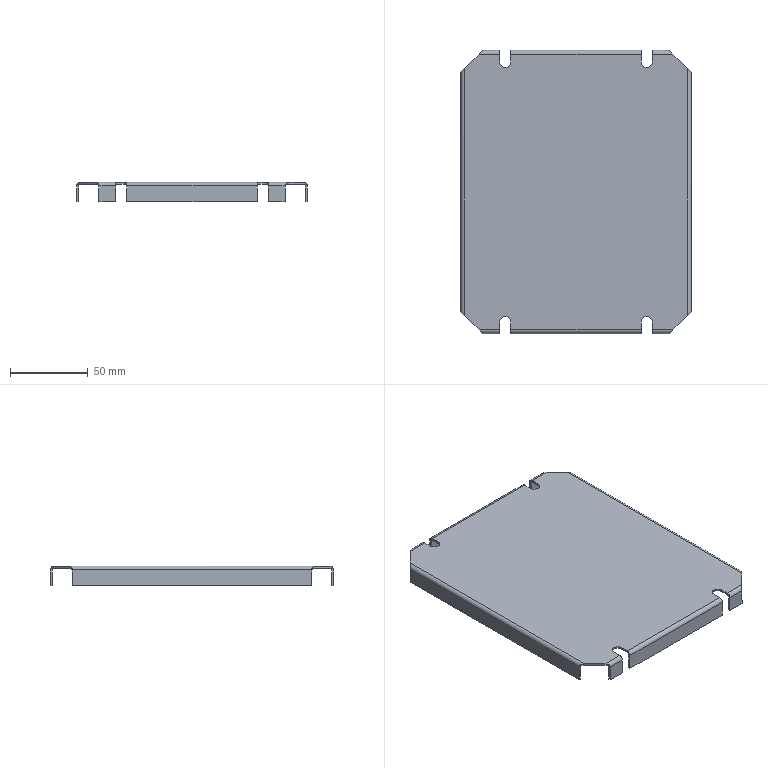Part | SolidWorks | features MoveFace 2, BaseBody 1 | 1 solid | 74 faces | box 148 x 182 x 12.6 mm | volume 38112 mm3 | plane 46 | cylinder 20 | spline 8 | commonest cylinder face diameters 2.4 x8 4.8 x8 7 x4